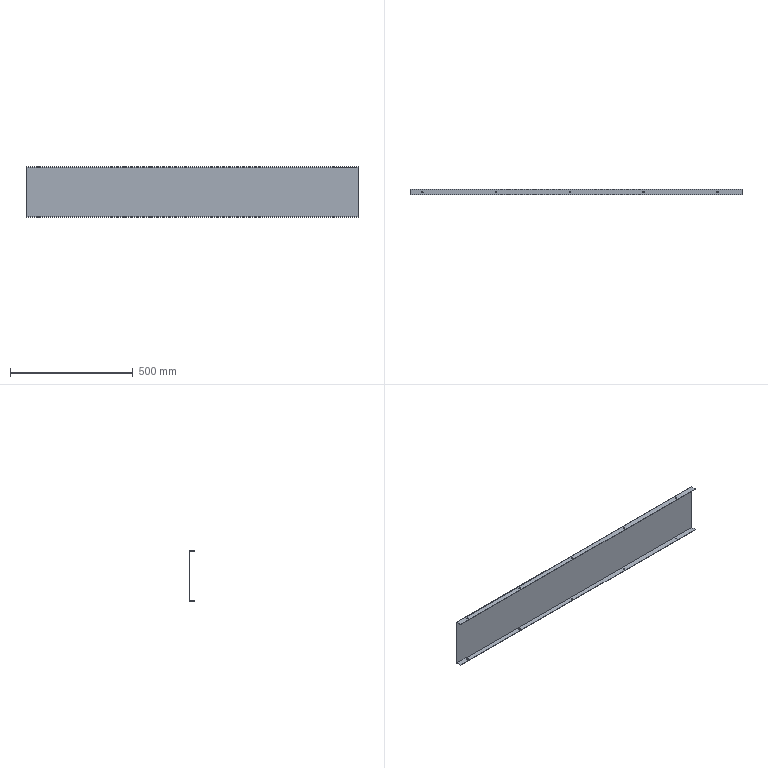Part | STEP file | 02-11 Belt line support plate | 1 solid | 30 faces | box 1350 x 22 x 204 mm | volume 495672 mm3 | cylinder 20 | plane 10 | commonest cylinder face diameters 6.2 x20